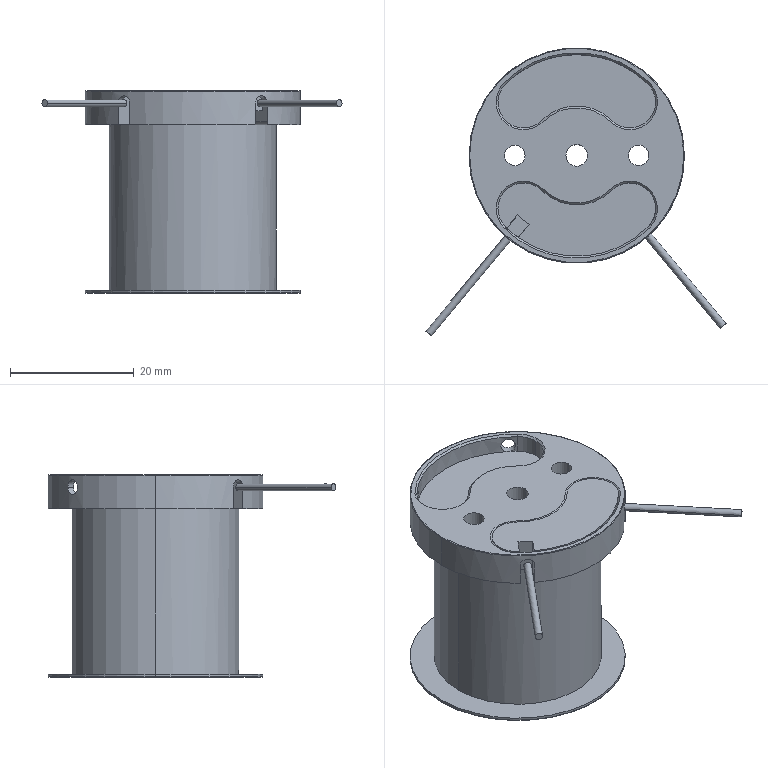Part | STEP file | COMPOUND | 3 solids | 74 faces | box 48.485 x 46.549 x 32.7 mm | volume 5431 mm3 | cylinder 41 | plane 19 | cone 10 | torus 4 | commonest cylinder face diameters 32.6 x7 2.4 x6 8.3 x6 1.2 x4 3.3 x4 34.8 x4